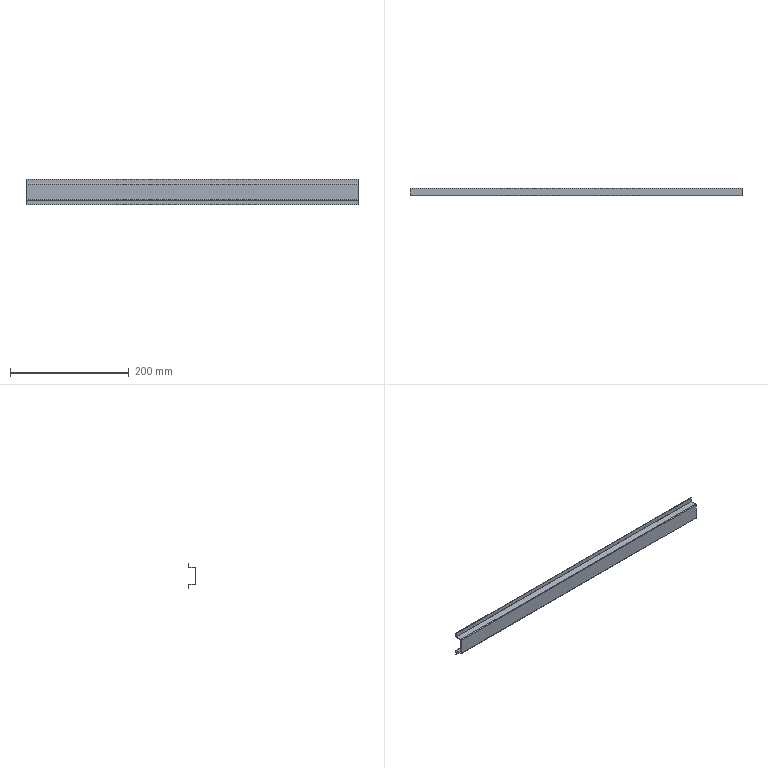Part | STEP file | HESS-408-70-15W-N-22-inner liner partition plate reinforcing rib | 1 solid | 22 faces | box 560 x 13 x 43 mm | volume 36943 mm3 | plane 14 | cylinder 8 | commonest cylinder face diameters 0.2 x4 2.2 x4